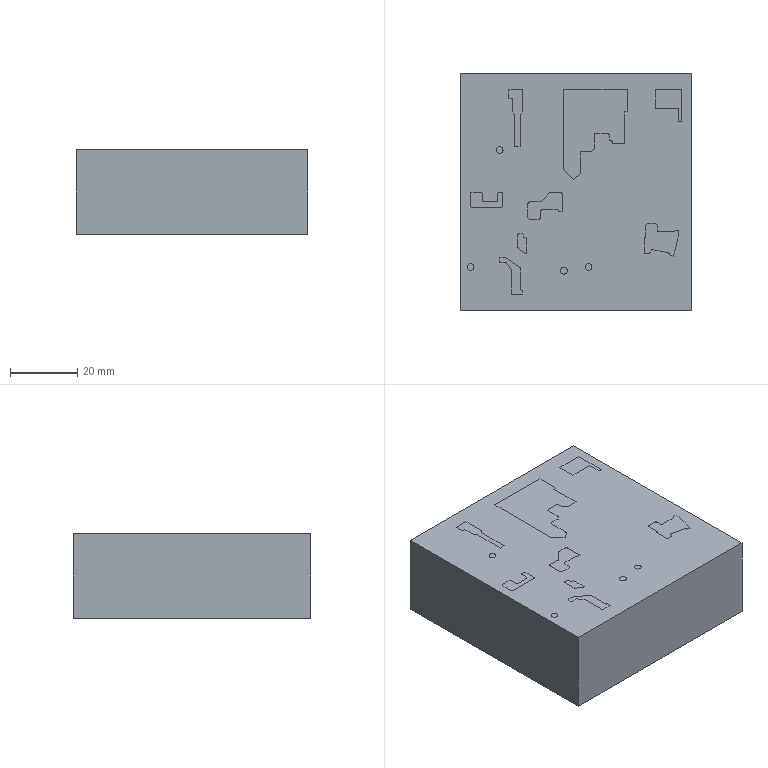Part | NX | features BREP 2 | 2 solids | 202 faces | box 68.723 x 70.502 x 25 mm | volume 221287 mm3 | plane 137 | cylinder 65 | commonest cylinder face diameters 1.1 x24 0.9 x20 3.1 x12 2 x3 188.149 x2 2.1 x1